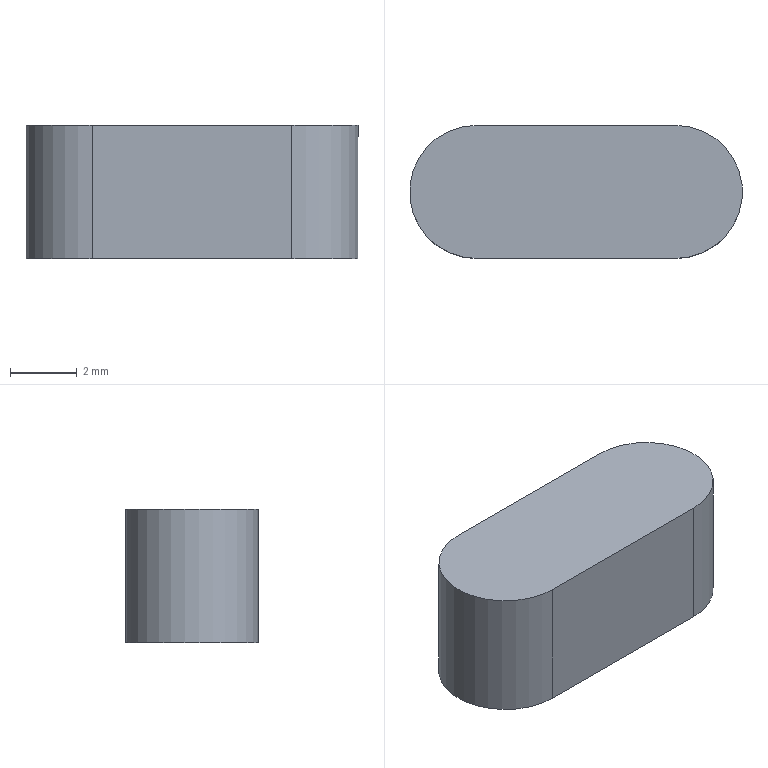Part | NX | features BREP 1 | 1 solid | 6 faces | box 10 x 4 x 4 mm | volume 146.265 mm3 | plane 4 | cylinder 2 | commonest cylinder face diameters 4 x2
STEP:
#1=CARTESIAN_POINT('',(-3.,2.,4.));
#2=VERTEX_POINT('',#1);
#3=CARTESIAN_POINT('',(-3.,-2.,4.));
#4=VERTEX_POINT('',#3);
#5=CARTESIAN_POINT('',(-3.,0.,4.));
#6=DIRECTION('',(0.,0.,1.));
#7=DIRECTION('',(1.,0.,0.));
#8=AXIS2_PLACEMENT_3D('',#5,#6,#7);
#9=CIRCLE('',#8,2.);
#10=EDGE_CURVE('',#2,#4,#9,.T.);
#11=ORIENTED_EDGE('',*,*,#10,.F.);
#12=CARTESIAN_POINT('',(-3.,2.,0.));
#13=VERTEX_POINT('',#12);
#14=CARTESIAN_POINT('',(-3.,2.,4.));
#15=DIRECTION('',(0.,0.,-1.));
#16=VECTOR('',#15,1000.);
#17=LINE('',#14,#16);
#18=EDGE_CURVE('',#2,#13,#17,.T.);
#19=ORIENTED_EDGE('',*,*,#18,.T.);
#20=CARTESIAN_POINT('',(-3.,-2.,0.));
#21=VERTEX_POINT('',#20);
#22=CARTESIAN_POINT('',(-3.,0.,0.));
#23=DIRECTION('',(0.,0.,1.));
#24=DIRECTION('',(1.,0.,0.));
#25=AXIS2_PLACEMENT_3D('',#22,#23,#24);
#26=CIRCLE('',#25,2.);
#27=EDGE_CURVE('',#13,#21,#26,.T.);
#28=ORIENTED_EDGE('',*,*,#27,.T.);
#29=CARTESIAN_POINT('',(-3.,-2.,4.));
#30=DIRECTION('',(0.,0.,-1.));
#31=VECTOR('',#30,1000.);
#32=LINE('',#29,#31);
#33=EDGE_CURVE('',#4,#21,#32,.T.);
#34=ORIENTED_EDGE('',*,*,#33,.F.);
#35=EDGE_LOOP('',(#11,#19,#28,#34));
#36=FACE_BOUND('',#35,.T.);
#37=CARTESIAN_POINT('',(-3.,0.,4.));
#38=DIRECTION('',(0.,0.,-1.));
#39=DIRECTION('',(-1.,0.,0.));
#40=AXIS2_PLACEMENT_3D('',#37,#38,#39);
#41=CYLINDRICAL_SURFACE('',#40,2.);
#42=ADVANCED_FACE('',(#36),#41,.T.);
#43=CARTESIAN_POINT('',(3.,-2.,0.));
#44=VERTEX_POINT('',#43);
#45=CARTESIAN_POINT('',(-3.,-2.,0.));
#46=DIRECTION('',(1.,0.,0.));
#47=VECTOR('',#46,1000.);
#48=LINE('',#45,#47);
#49=EDGE_CURVE('',#21,#44,#48,.T.);
#50=ORIENTED_EDGE('',*,*,#49,.T.);
#51=CARTESIAN_POINT('',(3.,-2.,4.));
#52=VERTEX_POINT('',#51);
#53=CARTESIAN_POINT('',(3.,-2.,4.));
#54=DIRECTION('',(0.,0.,-1.));
#55=VECTOR('',#54,1000.);
#56=LINE('',#53,#55);
#57=EDGE_CURVE('',#52,#44,#56,.T.);
#58=ORIENTED_EDGE('',*,*,#57,.F.);
#59=CARTESIAN_POINT('',(-3.,-2.,4.));
#60=DIRECTION('',(1.,0.,0.));
#61=VECTOR('',#60,1000.);
#62=LINE('',#59,#61);
#63=EDGE_CURVE('',#4,#52,#62,.T.);
#64=ORIENTED_EDGE('',*,*,#63,.F.);
#65=ORIENTED_EDGE('',*,*,#33,.T.);
#66=EDGE_LOOP('',(#50,#58,#64,#65));
#67=FACE_BOUND('',#66,.T.);
#68=CARTESIAN_POINT('',(-3.,-2.,4.));
#69=DIRECTION('',(0.,1.,0.));
#70=DIRECTION('',(-1.,0.,0.));
#71=AXIS2_PLACEMENT_3D('',#68,#69,#70);
#72=PLANE('',#71);
#73=ADVANCED_FACE('',(#67),#72,.F.);
#74=CARTESIAN_POINT('',(3.,2.,0.));
#75=VERTEX_POINT('',#74);
#76=CARTESIAN_POINT('',(3.,0.,0.));
#77=DIRECTION('',(0.,0.,1.));
#78=DIRECTION('',(1.,0.,0.));
#79=AXIS2_PLACEMENT_3D('',#76,#77,#78);
#80=CIRCLE('',#79,2.);
#81=EDGE_CURVE('',#44,#75,#80,.T.);
#82=ORIENTED_EDGE('',*,*,#81,.T.);
#83=CARTESIAN_POINT('',(3.,2.,4.));
#84=VERTEX_POINT('',#83);
#85=CARTESIAN_POINT('',(3.,2.,4.));
#86=DIRECTION('',(0.,0.,-1.));
#87=VECTOR('',#86,1000.);
#88=LINE('',#85,#87);
#89=EDGE_CURVE('',#84,#75,#88,.T.);
#90=ORIENTED_EDGE('',*,*,#89,.F.);
#91=CARTESIAN_POINT('',(3.,0.,4.));
#92=DIRECTION('',(0.,0.,1.));
#93=DIRECTION('',(1.,0.,0.));
#94=AXIS2_PLACEMENT_3D('',#91,#92,#93);
#95=CIRCLE('',#94,2.);
#96=EDGE_CURVE('',#52,#84,#95,.T.);
#97=ORIENTED_EDGE('',*,*,#96,.F.);
#98=ORIENTED_EDGE('',*,*,#57,.T.);
#99=EDGE_LOOP('',(#82,#90,#97,#98));
#100=FACE_BOUND('',#99,.T.);
#101=CARTESIAN_POINT('',(3.,0.,4.));
#102=DIRECTION('',(0.,0.,-1.));
#103=DIRECTION('',(-1.,0.,0.));
#104=AXIS2_PLACEMENT_3D('',#101,#102,#103);
#105=CYLINDRICAL_SURFACE('',#104,2.);
#106=ADVANCED_FACE('',(#100),#105,.T.);
#107=CARTESIAN_POINT('',(-3.,2.,0.));
#108=DIRECTION('',(-1.,0.,0.));
#109=VECTOR('',#108,1000.);
#110=LINE('',#107,#109);
#111=EDGE_CURVE('',#75,#13,#110,.T.);
#112=ORIENTED_EDGE('',*,*,#111,.T.);
#113=ORIENTED_EDGE('',*,*,#18,.F.);
#114=CARTESIAN_POINT('',(-3.,2.,4.));
#115=DIRECTION('',(-1.,0.,0.));
#116=VECTOR('',#115,1000.);
#117=LINE('',#114,#116);
#118=EDGE_CURVE('',#84,#2,#117,.T.);
#119=ORIENTED_EDGE('',*,*,#118,.F.);
#120=ORIENTED_EDGE('',*,*,#89,.T.);
#121=EDGE_LOOP('',(#112,#113,#119,#120));
#122=FACE_BOUND('',#121,.T.);
#123=CARTESIAN_POINT('',(-3.,2.,4.));
#124=DIRECTION('',(0.,-1.,0.));
#125=DIRECTION('',(0.,0.,-1.));
#126=AXIS2_PLACEMENT_3D('',#123,#124,#125);
#127=PLANE('',#126);
#128=ADVANCED_FACE('',(#122),#127,.F.);
#129=ORIENTED_EDGE('',*,*,#118,.T.);
#130=ORIENTED_EDGE('',*,*,#10,.T.);
#131=ORIENTED_EDGE('',*,*,#63,.T.);
#132=ORIENTED_EDGE('',*,*,#96,.T.);
#133=EDGE_LOOP('',(#129,#130,#131,#132));
#134=FACE_BOUND('',#133,.T.);
#135=CARTESIAN_POINT('',(-3.,0.,4.));
#136=DIRECTION('',(0.,0.,1.));
#137=DIRECTION('',(1.,0.,0.));
#138=AXIS2_PLACEMENT_3D('',#135,#136,#137);
#139=PLANE('',#138);
#140=ADVANCED_FACE('',(#134),#139,.T.);
#141=ORIENTED_EDGE('',*,*,#27,.F.);
#142=ORIENTED_EDGE('',*,*,#111,.F.);
#143=ORIENTED_EDGE('',*,*,#81,.F.);
#144=ORIENTED_EDGE('',*,*,#49,.F.);
#145=EDGE_LOOP('',(#141,#142,#143,#144));
#146=FACE_BOUND('',#145,.T.);
#147=CARTESIAN_POINT('',(-3.,0.,0.));
#148=DIRECTION('',(0.,0.,1.));
#149=DIRECTION('',(1.,0.,0.));
#150=AXIS2_PLACEMENT_3D('',#147,#148,#149);
#151=PLANE('',#150);
#152=ADVANCED_FACE('',(#146),#151,.F.);
#153=CLOSED_SHELL('',(#42,#73,#106,#128,#140,#152));
#154=MANIFOLD_SOLID_BREP('',#153);
#155=(LENGTH_UNIT()NAMED_UNIT(*)SI_UNIT(.MILLI.,.METRE.));
#156=UNCERTAINTY_MEASURE_WITH_UNIT(LENGTH_MEASURE(0.00001),#155,'','');
#157=(NAMED_UNIT(*)PLANE_ANGLE_UNIT()SI_UNIT($,.RADIAN.));
#158=(NAMED_UNIT(*)SI_UNIT($,.STERADIAN.)SOLID_ANGLE_UNIT());
#159=(GEOMETRIC_REPRESENTATION_CONTEXT(3)GLOBAL_UNCERTAINTY_ASSIGNED_CONTEXT((#156))GLOBAL_UNIT_ASSIGNED_CONTEXT((#155,#157,#158))REPRESENTATION_CONTEXT('',''));
#160=ADVANCED_BREP_SHAPE_REPRESENTATION('',(#154),#159);